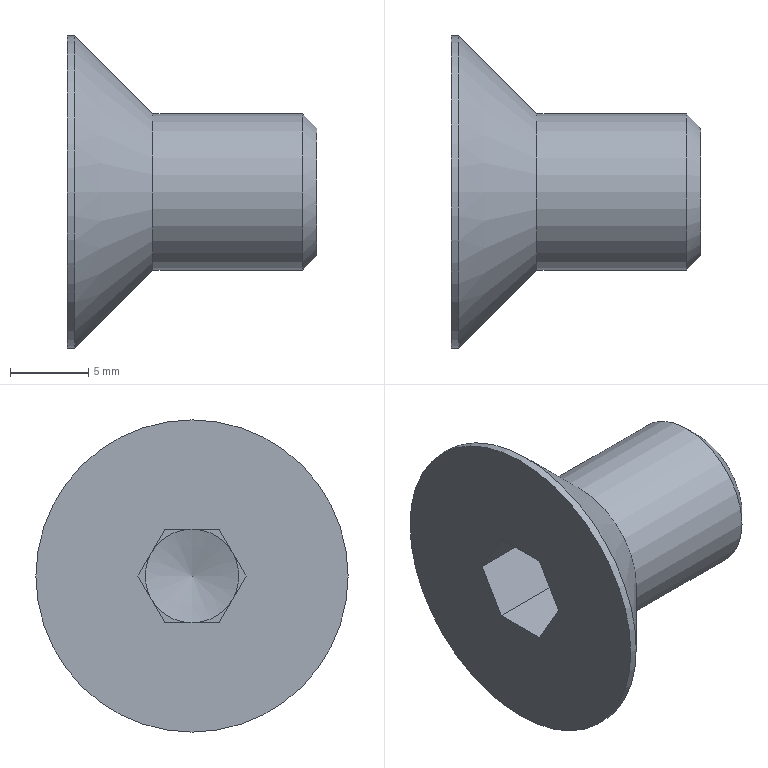Part | STEP file | FB10-16_ | 1 solid | 19 faces | box 16 x 20 x 20 mm | volume 1741 mm3 | plane 14 | cone 3 | cylinder 2 | commonest cylinder face diameters 10 x1 20 x1
STEP:
#1=CARTESIAN_POINT('',(0.,0.,-10.));
#2=VERTEX_POINT('',#1);
#3=CARTESIAN_POINT('',(0.,0.,10.));
#4=VERTEX_POINT('',#3);
#5=CARTESIAN_POINT('',(0.,0.,0.));
#6=DIRECTION('',(1.,0.,0.));
#7=DIRECTION('',(0.,0.,-1.));
#8=AXIS2_PLACEMENT_3D('',#5,#6,#7);
#9=CIRCLE('',#8,10.);
#10=EDGE_CURVE('',#2,#4,#9,.T.);
#11=ORIENTED_EDGE('',*,*,#10,.F.);
#12=CARTESIAN_POINT('',(0.,0.,0.));
#13=DIRECTION('',(1.,0.,0.));
#14=DIRECTION('',(0.,0.,-1.));
#15=AXIS2_PLACEMENT_3D('',#12,#13,#14);
#16=CIRCLE('',#15,10.);
#17=EDGE_CURVE('',#4,#2,#16,.T.);
#18=ORIENTED_EDGE('',*,*,#17,.F.);
#19=EDGE_LOOP('',(#11,#18));
#20=FACE_OUTER_BOUND('',#19,.T.);
#21=CARTESIAN_POINT('',(0.,-3.464,0.));
#22=VERTEX_POINT('',#21);
#23=CARTESIAN_POINT('',(0.,-1.732,-3.));
#24=VERTEX_POINT('',#23);
#25=CARTESIAN_POINT('',(0.,-3.464,0.));
#26=DIRECTION('',(0.,0.5,-0.866));
#27=VECTOR('',#26,1000.);
#28=LINE('',#25,#27);
#29=EDGE_CURVE('',#22,#24,#28,.T.);
#30=ORIENTED_EDGE('',*,*,#29,.T.);
#31=CARTESIAN_POINT('',(0.,1.732,-3.));
#32=VERTEX_POINT('',#31);
#33=CARTESIAN_POINT('',(0.,-1.732,-3.));
#34=DIRECTION('',(0.,1.,0.));
#35=VECTOR('',#34,1000.);
#36=LINE('',#33,#35);
#37=EDGE_CURVE('',#24,#32,#36,.T.);
#38=ORIENTED_EDGE('',*,*,#37,.T.);
#39=CARTESIAN_POINT('',(0.,3.464,0.));
#40=VERTEX_POINT('',#39);
#41=CARTESIAN_POINT('',(0.,1.732,-3.));
#42=DIRECTION('',(0.,0.5,0.866));
#43=VECTOR('',#42,1000.);
#44=LINE('',#41,#43);
#45=EDGE_CURVE('',#32,#40,#44,.T.);
#46=ORIENTED_EDGE('',*,*,#45,.T.);
#47=CARTESIAN_POINT('',(0.,1.732,3.));
#48=VERTEX_POINT('',#47);
#49=CARTESIAN_POINT('',(0.,3.464,0.));
#50=DIRECTION('',(0.,-0.5,0.866));
#51=VECTOR('',#50,1000.);
#52=LINE('',#49,#51);
#53=EDGE_CURVE('',#40,#48,#52,.T.);
#54=ORIENTED_EDGE('',*,*,#53,.T.);
#55=CARTESIAN_POINT('',(0.,-1.732,3.));
#56=VERTEX_POINT('',#55);
#57=CARTESIAN_POINT('',(0.,1.732,3.));
#58=DIRECTION('',(0.,-1.,0.));
#59=VECTOR('',#58,1000.);
#60=LINE('',#57,#59);
#61=EDGE_CURVE('',#48,#56,#60,.T.);
#62=ORIENTED_EDGE('',*,*,#61,.T.);
#63=CARTESIAN_POINT('',(0.,-1.732,3.));
#64=DIRECTION('',(0.,-0.5,-0.866));
#65=VECTOR('',#64,1000.);
#66=LINE('',#63,#65);
#67=EDGE_CURVE('',#56,#22,#66,.T.);
#68=ORIENTED_EDGE('',*,*,#67,.T.);
#69=EDGE_LOOP('',(#30,#38,#46,#54,#62,#68));
#70=FACE_BOUND('',#69,.T.);
#71=CARTESIAN_POINT('',(0.,0.,0.));
#72=DIRECTION('',(1.,0.,0.));
#73=DIRECTION('',(0.,0.,-1.));
#74=AXIS2_PLACEMENT_3D('',#71,#72,#73);
#75=PLANE('',#74);
#76=ADVANCED_FACE('',(#20,#70),#75,.F.);
#77=CARTESIAN_POINT('',(0.5,0.,-10.));
#78=VERTEX_POINT('',#77);
#79=CARTESIAN_POINT('',(0.5,0.,10.));
#80=VERTEX_POINT('',#79);
#81=CARTESIAN_POINT('',(0.5,0.,0.));
#82=DIRECTION('',(1.,0.,0.));
#83=DIRECTION('',(0.,0.,-1.));
#84=AXIS2_PLACEMENT_3D('',#81,#82,#83);
#85=CIRCLE('',#84,10.);
#86=EDGE_CURVE('',#78,#80,#85,.T.);
#87=ORIENTED_EDGE('',*,*,#86,.F.);
#88=CARTESIAN_POINT('',(0.5,0.,0.));
#89=DIRECTION('',(1.,0.,0.));
#90=DIRECTION('',(0.,0.,-1.));
#91=AXIS2_PLACEMENT_3D('',#88,#89,#90);
#92=CIRCLE('',#91,10.);
#93=EDGE_CURVE('',#80,#78,#92,.T.);
#94=ORIENTED_EDGE('',*,*,#93,.F.);
#95=CARTESIAN_POINT('',(16.,0.,10.));
#96=DIRECTION('',(-1.,0.,0.));
#97=VECTOR('',#96,10.);
#98=LINE('',#95,#97);
#99=EDGE_CURVE('',#80,#4,#98,.T.);
#100=ORIENTED_EDGE('',*,*,#99,.T.);
#101=ORIENTED_EDGE('',*,*,#17,.T.);
#102=ORIENTED_EDGE('',*,*,#10,.T.);
#103=ORIENTED_EDGE('',*,*,#99,.F.);
#104=EDGE_LOOP('',(#87,#94,#100,#101,#102,#103));
#105=FACE_OUTER_BOUND('',#104,.T.);
#106=CARTESIAN_POINT('',(16.,0.,0.));
#107=DIRECTION('',(1.,0.,0.));
#108=DIRECTION('',(0.,0.,-1.));
#109=AXIS2_PLACEMENT_3D('',#106,#107,#108);
#110=CYLINDRICAL_SURFACE('',#109,10.);
#111=ADVANCED_FACE('',(#105),#110,.T.);
#112=ORIENTED_EDGE('',*,*,#86,.T.);
#113=ORIENTED_EDGE('',*,*,#93,.T.);
#114=CARTESIAN_POINT('',(5.5,0.,-5.));
#115=VERTEX_POINT('',#114);
#116=CARTESIAN_POINT('',(0.5,0.,-10.));
#117=DIRECTION('',(0.7071,0.,0.7071));
#118=VECTOR('',#117,10.);
#119=LINE('',#116,#118);
#120=EDGE_CURVE('',#78,#115,#119,.T.);
#121=ORIENTED_EDGE('',*,*,#120,.T.);
#122=CARTESIAN_POINT('',(5.5,0.,5.));
#123=VERTEX_POINT('',#122);
#124=CARTESIAN_POINT('',(5.5,0.,0.));
#125=DIRECTION('',(1.,0.,0.));
#126=DIRECTION('',(0.,0.,-1.));
#127=AXIS2_PLACEMENT_3D('',#124,#125,#126);
#128=CIRCLE('',#127,5.);
#129=EDGE_CURVE('',#123,#115,#128,.T.);
#130=ORIENTED_EDGE('',*,*,#129,.F.);
#131=CARTESIAN_POINT('',(5.5,0.,0.));
#132=DIRECTION('',(1.,0.,0.));
#133=DIRECTION('',(0.,0.,-1.));
#134=AXIS2_PLACEMENT_3D('',#131,#132,#133);
#135=CIRCLE('',#134,5.);
#136=EDGE_CURVE('',#115,#123,#135,.T.);
#137=ORIENTED_EDGE('',*,*,#136,.F.);
#138=ORIENTED_EDGE('',*,*,#120,.F.);
#139=EDGE_LOOP('',(#112,#113,#121,#130,#137,#138));
#140=FACE_OUTER_BOUND('',#139,.T.);
#141=CARTESIAN_POINT('',(0.5,0.,0.));
#142=DIRECTION('',(-1.,0.,0.));
#143=DIRECTION('',(0.,0.,1.));
#144=AXIS2_PLACEMENT_3D('',#141,#142,#143);
#145=CONICAL_SURFACE('',#144,10.,0.7854);
#146=ADVANCED_FACE('',(#140),#145,.T.);
#147=CARTESIAN_POINT('',(15.08,0.,-5.));
#148=VERTEX_POINT('',#147);
#149=CARTESIAN_POINT('',(15.08,0.,5.));
#150=VERTEX_POINT('',#149);
#151=CARTESIAN_POINT('',(15.08,0.,0.));
#152=DIRECTION('',(1.,0.,0.));
#153=DIRECTION('',(0.,0.,-1.));
#154=AXIS2_PLACEMENT_3D('',#151,#152,#153);
#155=CIRCLE('',#154,5.);
#156=EDGE_CURVE('',#148,#150,#155,.T.);
#157=ORIENTED_EDGE('',*,*,#156,.F.);
#158=CARTESIAN_POINT('',(15.08,0.,0.));
#159=DIRECTION('',(1.,0.,0.));
#160=DIRECTION('',(0.,0.,-1.));
#161=AXIS2_PLACEMENT_3D('',#158,#159,#160);
#162=CIRCLE('',#161,5.);
#163=EDGE_CURVE('',#150,#148,#162,.T.);
#164=ORIENTED_EDGE('',*,*,#163,.F.);
#165=CARTESIAN_POINT('',(16.,0.,5.));
#166=DIRECTION('',(-1.,0.,0.));
#167=VECTOR('',#166,5.);
#168=LINE('',#165,#167);
#169=EDGE_CURVE('',#150,#123,#168,.T.);
#170=ORIENTED_EDGE('',*,*,#169,.T.);
#171=ORIENTED_EDGE('',*,*,#129,.T.);
#172=ORIENTED_EDGE('',*,*,#136,.T.);
#173=ORIENTED_EDGE('',*,*,#169,.F.);
#174=EDGE_LOOP('',(#157,#164,#170,#171,#172,#173));
#175=FACE_OUTER_BOUND('',#174,.T.);
#176=CARTESIAN_POINT('',(16.,0.,0.));
#177=DIRECTION('',(1.,0.,0.));
#178=DIRECTION('',(0.,0.,-1.));
#179=AXIS2_PLACEMENT_3D('',#176,#177,#178);
#180=CYLINDRICAL_SURFACE('',#179,5.);
#181=ADVANCED_FACE('',(#175),#180,.T.);
#182=ORIENTED_EDGE('',*,*,#156,.T.);
#183=ORIENTED_EDGE('',*,*,#163,.T.);
#184=CARTESIAN_POINT('',(16.,0.,-4.08));
#185=VERTEX_POINT('',#184);
#186=CARTESIAN_POINT('',(15.08,0.,-5.));
#187=DIRECTION('',(0.7071,0.,0.7071));
#188=VECTOR('',#187,5.);
#189=LINE('',#186,#188);
#190=EDGE_CURVE('',#148,#185,#189,.T.);
#191=ORIENTED_EDGE('',*,*,#190,.T.);
#192=CARTESIAN_POINT('',(16.,0.,0.));
#193=DIRECTION('',(1.,0.,0.));
#194=DIRECTION('',(0.,0.,-1.));
#195=AXIS2_PLACEMENT_3D('',#192,#193,#194);
#196=CIRCLE('',#195,4.08);
#197=EDGE_CURVE('',#185,#185,#196,.T.);
#198=ORIENTED_EDGE('',*,*,#197,.F.);
#199=ORIENTED_EDGE('',*,*,#190,.F.);
#200=EDGE_LOOP('',(#182,#183,#191,#198,#199));
#201=FACE_OUTER_BOUND('',#200,.T.);
#202=CARTESIAN_POINT('',(15.08,0.,0.));
#203=DIRECTION('',(-1.,0.,0.));
#204=DIRECTION('',(0.,0.,1.));
#205=AXIS2_PLACEMENT_3D('',#202,#203,#204);
#206=CONICAL_SURFACE('',#205,5.,0.7854);
#207=ADVANCED_FACE('',(#201),#206,.T.);
#208=ORIENTED_EDGE('',*,*,#197,.T.);
#209=EDGE_LOOP('',(#208));
#210=FACE_OUTER_BOUND('',#209,.T.);
#211=CARTESIAN_POINT('',(16.,4.08,0.));
#212=DIRECTION('',(-1.,0.,0.));
#213=DIRECTION('',(0.,0.,1.));
#214=AXIS2_PLACEMENT_3D('',#211,#212,#213);
#215=PLANE('',#214);
#216=ADVANCED_FACE('',(#210),#215,.F.);
#217=ORIENTED_EDGE('',*,*,#61,.F.);
#218=CARTESIAN_POINT('',(4.4,1.732,3.));
#219=VERTEX_POINT('',#218);
#220=CARTESIAN_POINT('',(4.4,1.732,3.));
#221=DIRECTION('',(-1.,0.,0.));
#222=VECTOR('',#221,1000.);
#223=LINE('',#220,#222);
#224=EDGE_CURVE('',#219,#48,#223,.T.);
#225=ORIENTED_EDGE('',*,*,#224,.F.);
#226=CARTESIAN_POINT('',(4.4,0.,3.));
#227=VERTEX_POINT('',#226);
#228=CARTESIAN_POINT('',(4.4,1.732,3.));
#229=DIRECTION('',(0.,-1.,0.));
#230=VECTOR('',#229,1000.);
#231=LINE('',#228,#230);
#232=EDGE_CURVE('',#219,#227,#231,.T.);
#233=ORIENTED_EDGE('',*,*,#232,.T.);
#234=CARTESIAN_POINT('',(4.4,-1.732,3.));
#235=VERTEX_POINT('',#234);
#236=CARTESIAN_POINT('',(4.4,1.732,3.));
#237=DIRECTION('',(0.,-1.,0.));
#238=VECTOR('',#237,1000.);
#239=LINE('',#236,#238);
#240=EDGE_CURVE('',#227,#235,#239,.T.);
#241=ORIENTED_EDGE('',*,*,#240,.T.);
#242=CARTESIAN_POINT('',(4.4,-1.732,3.));
#243=DIRECTION('',(-1.,0.,0.));
#244=VECTOR('',#243,1000.);
#245=LINE('',#242,#244);
#246=EDGE_CURVE('',#235,#56,#245,.T.);
#247=ORIENTED_EDGE('',*,*,#246,.T.);
#248=EDGE_LOOP('',(#217,#225,#233,#241,#247));
#249=FACE_OUTER_BOUND('',#248,.T.);
#250=CARTESIAN_POINT('',(4.4,1.732,3.));
#251=DIRECTION('',(0.,0.,-1.));
#252=DIRECTION('',(-1.,0.,0.));
#253=AXIS2_PLACEMENT_3D('',#250,#251,#252);
#254=PLANE('',#253);
#255=ADVANCED_FACE('',(#249),#254,.T.);
#256=ORIENTED_EDGE('',*,*,#67,.F.);
#257=ORIENTED_EDGE('',*,*,#246,.F.);
#258=CARTESIAN_POINT('',(4.4,-2.598,1.5));
#259=VERTEX_POINT('',#258);
#260=CARTESIAN_POINT('',(4.4,-1.732,3.));
#261=DIRECTION('',(0.,-0.5,-0.866));
#262=VECTOR('',#261,1000.);
#263=LINE('',#260,#262);
#264=EDGE_CURVE('',#235,#259,#263,.T.);
#265=ORIENTED_EDGE('',*,*,#264,.T.);
#266=CARTESIAN_POINT('',(4.4,-3.464,0.));
#267=VERTEX_POINT('',#266);
#268=CARTESIAN_POINT('',(4.4,-1.732,3.));
#269=DIRECTION('',(0.,-0.5,-0.866));
#270=VECTOR('',#269,1000.);
#271=LINE('',#268,#270);
#272=EDGE_CURVE('',#259,#267,#271,.T.);
#273=ORIENTED_EDGE('',*,*,#272,.T.);
#274=CARTESIAN_POINT('',(4.4,-3.464,0.));
#275=DIRECTION('',(-1.,0.,0.));
#276=VECTOR('',#275,1000.);
#277=LINE('',#274,#276);
#278=EDGE_CURVE('',#267,#22,#277,.T.);
#279=ORIENTED_EDGE('',*,*,#278,.T.);
#280=EDGE_LOOP('',(#256,#257,#265,#273,#279));
#281=FACE_OUTER_BOUND('',#280,.T.);
#282=CARTESIAN_POINT('',(4.4,-1.732,3.));
#283=DIRECTION('',(0.,0.866,-0.5));
#284=DIRECTION('',(0.,0.5,0.866));
#285=AXIS2_PLACEMENT_3D('',#282,#283,#284);
#286=PLANE('',#285);
#287=ADVANCED_FACE('',(#281),#286,.T.);
#288=ORIENTED_EDGE('',*,*,#29,.F.);
#289=ORIENTED_EDGE('',*,*,#278,.F.);
#290=CARTESIAN_POINT('',(4.4,-2.598,-1.5));
#291=VERTEX_POINT('',#290);
#292=CARTESIAN_POINT('',(4.4,-3.464,0.));
#293=DIRECTION('',(0.,0.5,-0.866));
#294=VECTOR('',#293,1000.);
#295=LINE('',#292,#294);
#296=EDGE_CURVE('',#267,#291,#295,.T.);
#297=ORIENTED_EDGE('',*,*,#296,.T.);
#298=CARTESIAN_POINT('',(4.4,-1.732,-3.));
#299=VERTEX_POINT('',#298);
#300=CARTESIAN_POINT('',(4.4,-3.464,0.));
#301=DIRECTION('',(0.,0.5,-0.866));
#302=VECTOR('',#301,1000.);
#303=LINE('',#300,#302);
#304=EDGE_CURVE('',#291,#299,#303,.T.);
#305=ORIENTED_EDGE('',*,*,#304,.T.);
#306=CARTESIAN_POINT('',(4.4,-1.732,-3.));
#307=DIRECTION('',(-1.,0.,0.));
#308=VECTOR('',#307,1000.);
#309=LINE('',#306,#308);
#310=EDGE_CURVE('',#299,#24,#309,.T.);
#311=ORIENTED_EDGE('',*,*,#310,.T.);
#312=EDGE_LOOP('',(#288,#289,#297,#305,#311));
#313=FACE_OUTER_BOUND('',#312,.T.);
#314=CARTESIAN_POINT('',(4.4,-3.464,0.));
#315=DIRECTION('',(0.,0.866,0.5));
#316=DIRECTION('',(0.,-0.5,0.866));
#317=AXIS2_PLACEMENT_3D('',#314,#315,#316);
#318=PLANE('',#317);
#319=ADVANCED_FACE('',(#313),#318,.T.);
#320=ORIENTED_EDGE('',*,*,#37,.F.);
#321=ORIENTED_EDGE('',*,*,#310,.F.);
#322=CARTESIAN_POINT('',(4.4,0.,-3.));
#323=VERTEX_POINT('',#322);
#324=CARTESIAN_POINT('',(4.4,-1.732,-3.));
#325=DIRECTION('',(0.,1.,0.));
#326=VECTOR('',#325,1000.);
#327=LINE('',#324,#326);
#328=EDGE_CURVE('',#299,#323,#327,.T.);
#329=ORIENTED_EDGE('',*,*,#328,.T.);
#330=CARTESIAN_POINT('',(4.4,1.732,-3.));
#331=VERTEX_POINT('',#330);
#332=CARTESIAN_POINT('',(4.4,-1.732,-3.));
#333=DIRECTION('',(0.,1.,0.));
#334=VECTOR('',#333,1000.);
#335=LINE('',#332,#334);
#336=EDGE_CURVE('',#323,#331,#335,.T.);
#337=ORIENTED_EDGE('',*,*,#336,.T.);
#338=CARTESIAN_POINT('',(4.4,1.732,-3.));
#339=DIRECTION('',(-1.,0.,0.));
#340=VECTOR('',#339,1000.);
#341=LINE('',#338,#340);
#342=EDGE_CURVE('',#331,#32,#341,.T.);
#343=ORIENTED_EDGE('',*,*,#342,.T.);
#344=EDGE_LOOP('',(#320,#321,#329,#337,#343));
#345=FACE_OUTER_BOUND('',#344,.T.);
#346=CARTESIAN_POINT('',(4.4,-1.732,-3.));
#347=DIRECTION('',(0.,0.,1.));
#348=DIRECTION('',(1.,0.,0.));
#349=AXIS2_PLACEMENT_3D('',#346,#347,#348);
#350=PLANE('',#349);
#351=ADVANCED_FACE('',(#345),#350,.T.);
#352=ORIENTED_EDGE('',*,*,#45,.F.);
#353=ORIENTED_EDGE('',*,*,#342,.F.);
#354=CARTESIAN_POINT('',(4.4,2.598,-1.5));
#355=VERTEX_POINT('',#354);
#356=CARTESIAN_POINT('',(4.4,1.732,-3.));
#357=DIRECTION('',(0.,0.5,0.866));
#358=VECTOR('',#357,1000.);
#359=LINE('',#356,#358);
#360=EDGE_CURVE('',#331,#355,#359,.T.);
#361=ORIENTED_EDGE('',*,*,#360,.T.);
#362=CARTESIAN_POINT('',(4.4,3.464,0.));
#363=VERTEX_POINT('',#362);
#364=CARTESIAN_POINT('',(4.4,1.732,-3.));
#365=DIRECTION('',(0.,0.5,0.866));
#366=VECTOR('',#365,1000.);
#367=LINE('',#364,#366);
#368=EDGE_CURVE('',#355,#363,#367,.T.);
#369=ORIENTED_EDGE('',*,*,#368,.T.);
#370=CARTESIAN_POINT('',(4.4,3.464,0.));
#371=DIRECTION('',(-1.,0.,0.));
#372=VECTOR('',#371,1000.);
#373=LINE('',#370,#372);
#374=EDGE_CURVE('',#363,#40,#373,.T.);
#375=ORIENTED_EDGE('',*,*,#374,.T.);
#376=EDGE_LOOP('',(#352,#353,#361,#369,#375));
#377=FACE_OUTER_BOUND('',#376,.T.);
#378=CARTESIAN_POINT('',(4.4,1.732,-3.));
#379=DIRECTION('',(0.,-0.866,0.5));
#380=DIRECTION('',(0.,-0.5,-0.866));
#381=AXIS2_PLACEMENT_3D('',#378,#379,#380);
#382=PLANE('',#381);
#383=ADVANCED_FACE('',(#377),#382,.T.);
#384=ORIENTED_EDGE('',*,*,#53,.F.);
#385=ORIENTED_EDGE('',*,*,#374,.F.);
#386=CARTESIAN_POINT('',(4.4,2.598,1.5));
#387=VERTEX_POINT('',#386);
#388=CARTESIAN_POINT('',(4.4,3.464,0.));
#389=DIRECTION('',(0.,-0.5,0.866));
#390=VECTOR('',#389,1000.);
#391=LINE('',#388,#390);
#392=EDGE_CURVE('',#363,#387,#391,.T.);
#393=ORIENTED_EDGE('',*,*,#392,.T.);
#394=CARTESIAN_POINT('',(4.4,3.464,0.));
#395=DIRECTION('',(0.,-0.5,0.866));
#396=VECTOR('',#395,1000.);
#397=LINE('',#394,#396);
#398=EDGE_CURVE('',#387,#219,#397,.T.);
#399=ORIENTED_EDGE('',*,*,#398,.T.);
#400=ORIENTED_EDGE('',*,*,#224,.T.);
#401=EDGE_LOOP('',(#384,#385,#393,#399,#400));
#402=FACE_OUTER_BOUND('',#401,.T.);
#403=CARTESIAN_POINT('',(4.4,3.464,0.));
#404=DIRECTION('',(0.,-0.866,-0.5));
#405=DIRECTION('',(0.,0.5,-0.866));
#406=AXIS2_PLACEMENT_3D('',#403,#404,#405);
#407=PLANE('',#406);
#408=ADVANCED_FACE('',(#402),#407,.T.);
#409=CARTESIAN_POINT('',(4.4,0.,0.));
#410=DIRECTION('',(1.,0.,0.));
#411=DIRECTION('',(0.,0.,-1.));
#412=AXIS2_PLACEMENT_3D('',#409,#410,#411);
#413=CIRCLE('',#412,3.);
#414=EDGE_CURVE('',#323,#355,#413,.T.);
#415=ORIENTED_EDGE('',*,*,#414,.T.);
#416=ORIENTED_EDGE('',*,*,#360,.F.);
#417=ORIENTED_EDGE('',*,*,#336,.F.);
#418=EDGE_LOOP('',(#415,#416,#417));
#419=FACE_OUTER_BOUND('',#418,.T.);
#420=CARTESIAN_POINT('',(4.4,0.,0.));
#421=DIRECTION('',(1.,0.,0.));
#422=DIRECTION('',(0.,0.,-1.));
#423=AXIS2_PLACEMENT_3D('',#420,#421,#422);
#424=PLANE('',#423);
#425=ADVANCED_FACE('',(#419),#424,.F.);
#426=ORIENTED_EDGE('',*,*,#368,.F.);
#427=CARTESIAN_POINT('',(4.4,0.,0.));
#428=DIRECTION('',(1.,0.,0.));
#429=DIRECTION('',(0.,0.,-1.));
#430=AXIS2_PLACEMENT_3D('',#427,#428,#429);
#431=CIRCLE('',#430,3.);
#432=EDGE_CURVE('',#355,#387,#431,.T.);
#433=ORIENTED_EDGE('',*,*,#432,.T.);
#434=ORIENTED_EDGE('',*,*,#392,.F.);
#435=EDGE_LOOP('',(#426,#433,#434));
#436=FACE_OUTER_BOUND('',#435,.T.);
#437=CARTESIAN_POINT('',(4.4,0.,0.));
#438=DIRECTION('',(1.,0.,0.));
#439=DIRECTION('',(0.,0.,-1.));
#440=AXIS2_PLACEMENT_3D('',#437,#438,#439);
#441=PLANE('',#440);
#442=ADVANCED_FACE('',(#436),#441,.F.);
#443=CARTESIAN_POINT('',(4.4,0.,0.));
#444=DIRECTION('',(1.,0.,0.));
#445=DIRECTION('',(0.,0.,-1.));
#446=AXIS2_PLACEMENT_3D('',#443,#444,#445);
#447=CIRCLE('',#446,3.);
#448=EDGE_CURVE('',#387,#227,#447,.T.);
#449=ORIENTED_EDGE('',*,*,#448,.T.);
#450=ORIENTED_EDGE('',*,*,#232,.F.);
#451=ORIENTED_EDGE('',*,*,#398,.F.);
#452=EDGE_LOOP('',(#449,#450,#451));
#453=FACE_OUTER_BOUND('',#452,.T.);
#454=CARTESIAN_POINT('',(4.4,0.,0.));
#455=DIRECTION('',(1.,0.,0.));
#456=DIRECTION('',(0.,0.,-1.));
#457=AXIS2_PLACEMENT_3D('',#454,#455,#456);
#458=PLANE('',#457);
#459=ADVANCED_FACE('',(#453),#458,.F.);
#460=CARTESIAN_POINT('',(4.4,0.,0.));
#461=DIRECTION('',(1.,0.,0.));
#462=DIRECTION('',(0.,0.,-1.));
#463=AXIS2_PLACEMENT_3D('',#460,#461,#462);
#464=CIRCLE('',#463,3.);
#465=EDGE_CURVE('',#227,#259,#464,.T.);
#466=ORIENTED_EDGE('',*,*,#465,.T.);
#467=ORIENTED_EDGE('',*,*,#264,.F.);
#468=ORIENTED_EDGE('',*,*,#240,.F.);
#469=EDGE_LOOP('',(#466,#467,#468));
#470=FACE_OUTER_BOUND('',#469,.T.);
#471=CARTESIAN_POINT('',(4.4,0.,0.));
#472=DIRECTION('',(1.,0.,0.));
#473=DIRECTION('',(0.,0.,-1.));
#474=AXIS2_PLACEMENT_3D('',#471,#472,#473);
#475=PLANE('',#474);
#476=ADVANCED_FACE('',(#470),#475,.F.);
#477=CARTESIAN_POINT('',(4.4,0.,0.));
#478=DIRECTION('',(1.,0.,0.));
#479=DIRECTION('',(0.,0.,-1.));
#480=AXIS2_PLACEMENT_3D('',#477,#478,#479);
#481=CIRCLE('',#480,3.);
#482=EDGE_CURVE('',#259,#291,#481,.T.);
#483=ORIENTED_EDGE('',*,*,#482,.T.);
#484=ORIENTED_EDGE('',*,*,#296,.F.);
#485=ORIENTED_EDGE('',*,*,#272,.F.);
#486=EDGE_LOOP('',(#483,#484,#485));
#487=FACE_OUTER_BOUND('',#486,.T.);
#488=CARTESIAN_POINT('',(4.4,0.,0.));
#489=DIRECTION('',(1.,0.,0.));
#490=DIRECTION('',(0.,0.,-1.));
#491=AXIS2_PLACEMENT_3D('',#488,#489,#490);
#492=PLANE('',#491);
#493=ADVANCED_FACE('',(#487),#492,.F.);
#494=CARTESIAN_POINT('',(4.4,0.,0.));
#495=DIRECTION('',(1.,0.,0.));
#496=DIRECTION('',(0.,0.,-1.));
#497=AXIS2_PLACEMENT_3D('',#494,#495,#496);
#498=CIRCLE('',#497,3.);
#499=EDGE_CURVE('',#291,#323,#498,.T.);
#500=ORIENTED_EDGE('',*,*,#499,.T.);
#501=ORIENTED_EDGE('',*,*,#328,.F.);
#502=ORIENTED_EDGE('',*,*,#304,.F.);
#503=EDGE_LOOP('',(#500,#501,#502));
#504=FACE_OUTER_BOUND('',#503,.T.);
#505=CARTESIAN_POINT('',(4.4,0.,0.));
#506=DIRECTION('',(1.,0.,0.));
#507=DIRECTION('',(0.,0.,-1.));
#508=AXIS2_PLACEMENT_3D('',#505,#506,#507);
#509=PLANE('',#508);
#510=ADVANCED_FACE('',(#504),#509,.F.);
#511=CARTESIAN_POINT('',(5.204,0.,0.));
#512=VERTEX_POINT('',#511);
#513=CARTESIAN_POINT('',(4.4,0.,-3.));
#514=DIRECTION('',(-0.2588,0.,-0.9659));
#515=VECTOR('',#514,3.);
#516=LINE('',#513,#515);
#517=EDGE_CURVE('',#512,#323,#516,.T.);
#518=ORIENTED_EDGE('',*,*,#517,.T.);
#519=ORIENTED_EDGE('',*,*,#499,.F.);
#520=ORIENTED_EDGE('',*,*,#482,.F.);
#521=ORIENTED_EDGE('',*,*,#465,.F.);
#522=ORIENTED_EDGE('',*,*,#448,.F.);
#523=ORIENTED_EDGE('',*,*,#432,.F.);
#524=ORIENTED_EDGE('',*,*,#414,.F.);
#525=ORIENTED_EDGE('',*,*,#517,.F.);
#526=EDGE_LOOP('',(#518,#519,#520,#521,#522,#523,#524,#525));
#527=FACE_OUTER_BOUND('',#526,.T.);
#528=CARTESIAN_POINT('',(4.4,0.,0.));
#529=DIRECTION('',(-1.,0.,0.));
#530=DIRECTION('',(0.,0.,1.));
#531=AXIS2_PLACEMENT_3D('',#528,#529,#530);
#532=CONICAL_SURFACE('',#531,3.,1.309);
#533=ADVANCED_FACE('',(#527),#532,.F.);
#534=CLOSED_SHELL('',(#76,#111,#146,#181,#207,#216,#255,#287,#319,#351,#383,#408,#425,#442,#459,#476,#493,#510,#533));
#535=MANIFOLD_SOLID_BREP('',#534);
#536=(LENGTH_UNIT()NAMED_UNIT(*)SI_UNIT(.MILLI.,.METRE.));
#537=UNCERTAINTY_MEASURE_WITH_UNIT(LENGTH_MEASURE(0.01),#536,'','');
#538=(NAMED_UNIT(*)PLANE_ANGLE_UNIT()SI_UNIT($,.RADIAN.));
#539=(NAMED_UNIT(*)SI_UNIT($,.STERADIAN.)SOLID_ANGLE_UNIT());
#540=(GEOMETRIC_REPRESENTATION_CONTEXT(3)GLOBAL_UNCERTAINTY_ASSIGNED_CONTEXT((#537))GLOBAL_UNIT_ASSIGNED_CONTEXT((#536,#538,#539))REPRESENTATION_CONTEXT('',''));
#541=ADVANCED_BREP_SHAPE_REPRESENTATION('',(#535),#540);